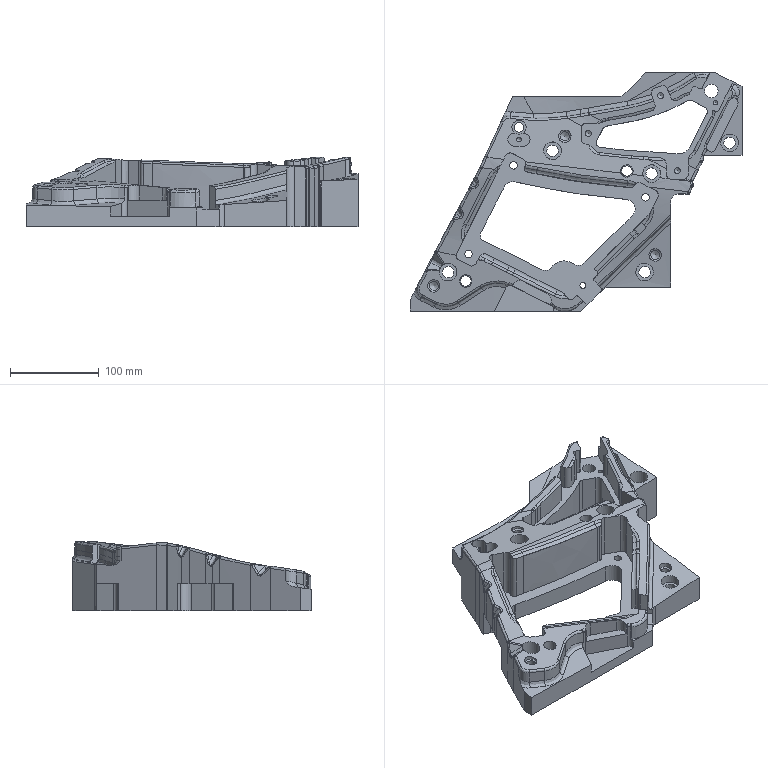Part | STEP file | gslz 2016.10.28-13_id522_x_t | 1 solid | 483 faces | box 375 x 269 x 78.578 mm | volume 2153207 mm3 | spline 238 | cylinder 105 | plane 99 | other 29 | cone 11 | sphere 1 | commonest cylinder face diameters 12 x26 18 x14 6 x8 8 x7 20 x7 13 x5